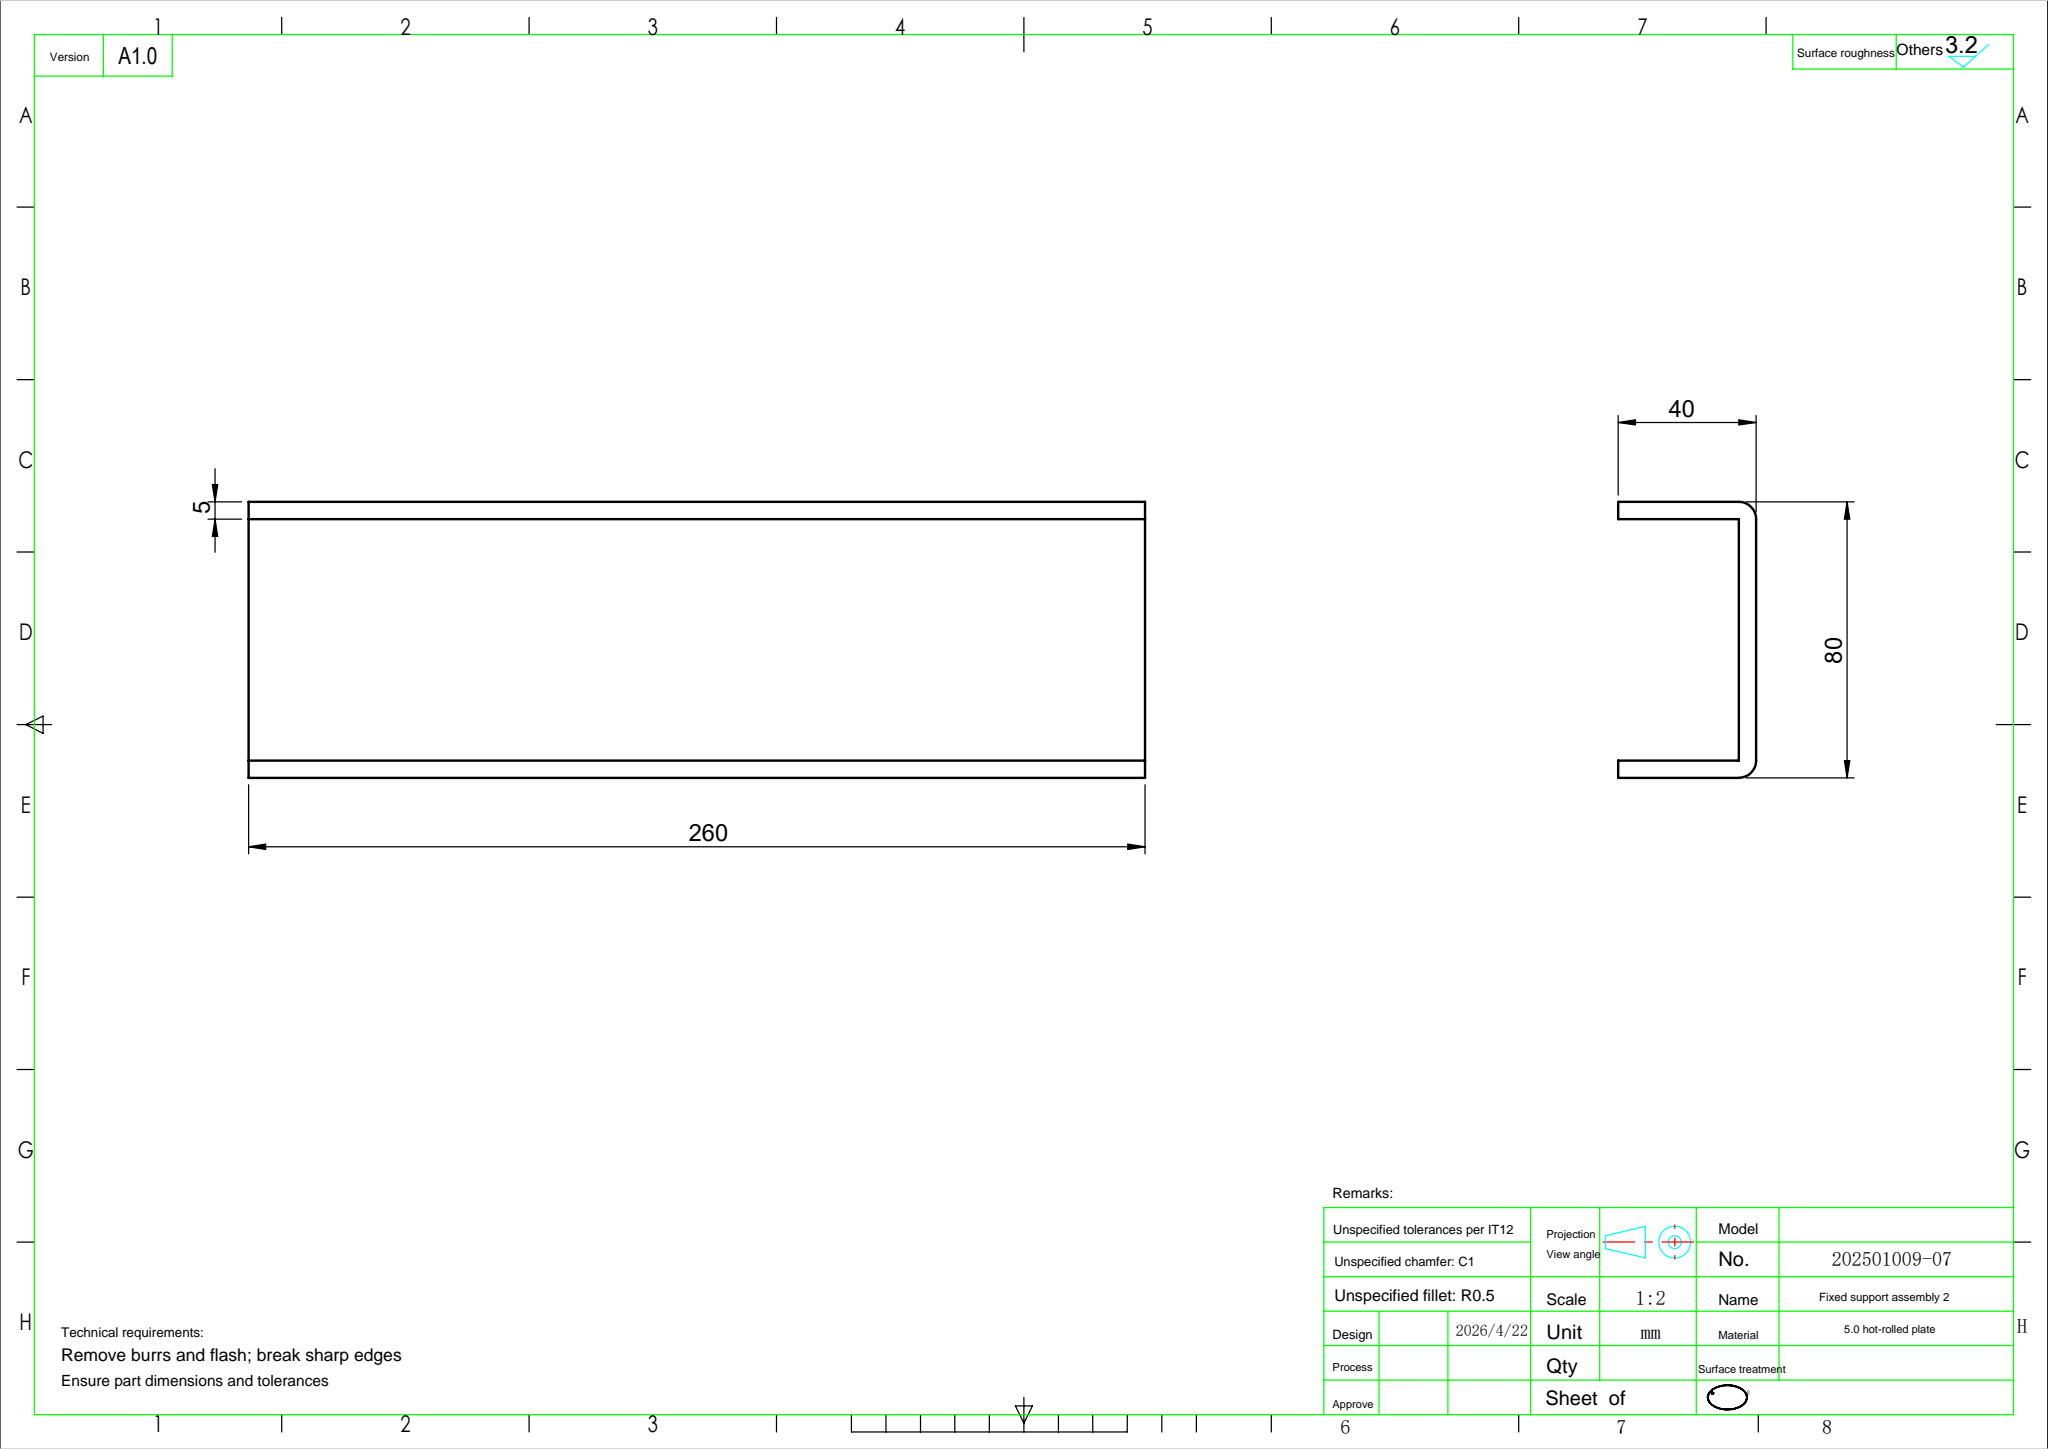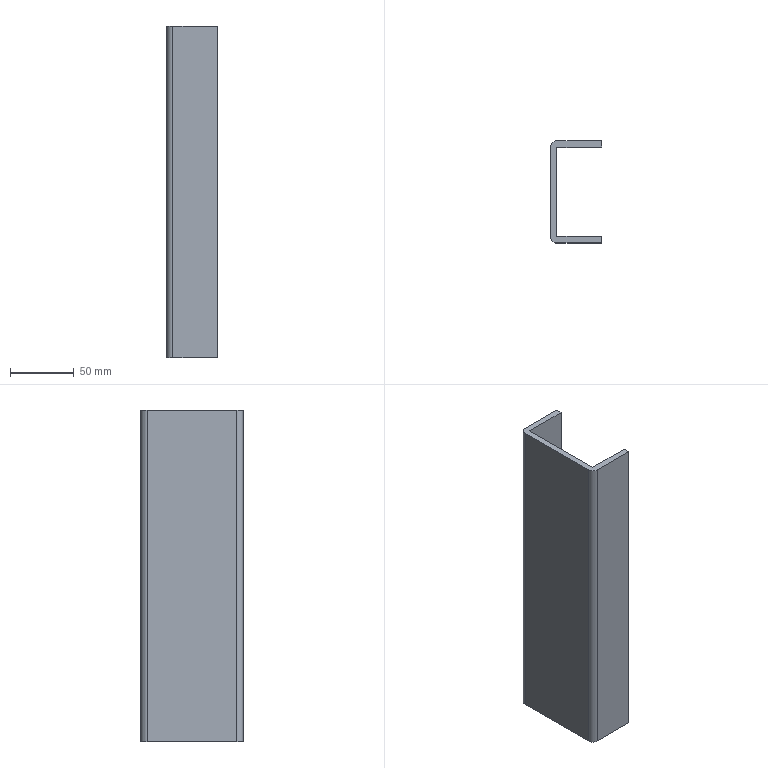Part | SolidWorks | features ExtruThin 1, Fillet 1 | 1 solid | 12 faces | box 40 x 80 x 260 mm | volume 192210 mm3 | plane 10 | cylinder 2 | commonest cylinder face diameters 10 x2
STEP:
#1=CARTESIAN_POINT('',(5.,35.,0.));
#2=VERTEX_POINT('',#1);
#3=CARTESIAN_POINT('',(40.,35.,0.));
#4=VERTEX_POINT('',#3);
#5=CARTESIAN_POINT('',(0.,35.,0.));
#6=DIRECTION('',(1.,0.,0.));
#7=VECTOR('',#6,1000.);
#8=LINE('',#5,#7);
#9=EDGE_CURVE('',#2,#4,#8,.T.);
#10=ORIENTED_EDGE('',*,*,#9,.T.);
#11=CARTESIAN_POINT('',(40.,35.,260.));
#12=VERTEX_POINT('',#11);
#13=CARTESIAN_POINT('',(40.,35.,260.));
#14=DIRECTION('',(0.,0.,-1.));
#15=VECTOR('',#14,1000.);
#16=LINE('',#13,#15);
#17=EDGE_CURVE('',#12,#4,#16,.T.);
#18=ORIENTED_EDGE('',*,*,#17,.F.);
#19=CARTESIAN_POINT('',(5.,35.,260.));
#20=VERTEX_POINT('',#19);
#21=CARTESIAN_POINT('',(0.,35.,260.));
#22=DIRECTION('',(1.,0.,0.));
#23=VECTOR('',#22,1000.);
#24=LINE('',#21,#23);
#25=EDGE_CURVE('',#20,#12,#24,.T.);
#26=ORIENTED_EDGE('',*,*,#25,.F.);
#27=CARTESIAN_POINT('',(5.,35.,260.));
#28=DIRECTION('',(0.,0.,-1.));
#29=VECTOR('',#28,1000.);
#30=LINE('',#27,#29);
#31=EDGE_CURVE('',#20,#2,#30,.T.);
#32=ORIENTED_EDGE('',*,*,#31,.T.);
#33=EDGE_LOOP('',(#10,#18,#26,#32));
#34=FACE_OUTER_BOUND('',#33,.T.);
#35=CARTESIAN_POINT('',(0.,35.,260.));
#36=DIRECTION('',(0.,1.,0.));
#37=DIRECTION('',(0.,0.,1.));
#38=AXIS2_PLACEMENT_3D('',#35,#36,#37);
#39=PLANE('',#38);
#40=ADVANCED_FACE('',(#34),#39,.F.);
#41=CARTESIAN_POINT('',(40.,40.,0.));
#42=VERTEX_POINT('',#41);
#43=CARTESIAN_POINT('',(40.,40.,0.));
#44=DIRECTION('',(0.,-1.,0.));
#45=VECTOR('',#44,1000.);
#46=LINE('',#43,#45);
#47=EDGE_CURVE('',#42,#4,#46,.T.);
#48=ORIENTED_EDGE('',*,*,#47,.F.);
#49=CARTESIAN_POINT('',(40.,40.,260.));
#50=VERTEX_POINT('',#49);
#51=CARTESIAN_POINT('',(40.,40.,260.));
#52=DIRECTION('',(0.,0.,-1.));
#53=VECTOR('',#52,1000.);
#54=LINE('',#51,#53);
#55=EDGE_CURVE('',#50,#42,#54,.T.);
#56=ORIENTED_EDGE('',*,*,#55,.F.);
#57=CARTESIAN_POINT('',(40.,40.,260.));
#58=DIRECTION('',(0.,-1.,0.));
#59=VECTOR('',#58,1000.);
#60=LINE('',#57,#59);
#61=EDGE_CURVE('',#50,#12,#60,.T.);
#62=ORIENTED_EDGE('',*,*,#61,.T.);
#63=ORIENTED_EDGE('',*,*,#17,.T.);
#64=EDGE_LOOP('',(#48,#56,#62,#63));
#65=FACE_OUTER_BOUND('',#64,.T.);
#66=CARTESIAN_POINT('',(40.,40.,260.));
#67=DIRECTION('',(1.,0.,0.));
#68=DIRECTION('',(0.,0.,-1.));
#69=AXIS2_PLACEMENT_3D('',#66,#67,#68);
#70=PLANE('',#69);
#71=ADVANCED_FACE('',(#65),#70,.T.);
#72=CARTESIAN_POINT('',(5.,40.,0.));
#73=VERTEX_POINT('',#72);
#74=CARTESIAN_POINT('',(0.,40.,0.));
#75=DIRECTION('',(1.,0.,0.));
#76=VECTOR('',#75,1000.);
#77=LINE('',#74,#76);
#78=EDGE_CURVE('',#73,#42,#77,.T.);
#79=ORIENTED_EDGE('',*,*,#78,.F.);
#80=CARTESIAN_POINT('',(5.,40.,260.));
#81=VERTEX_POINT('',#80);
#82=CARTESIAN_POINT('',(5.,40.,260.));
#83=DIRECTION('',(0.,0.,1.));
#84=VECTOR('',#83,1000.);
#85=LINE('',#82,#84);
#86=EDGE_CURVE('',#73,#81,#85,.T.);
#87=ORIENTED_EDGE('',*,*,#86,.T.);
#88=CARTESIAN_POINT('',(0.,40.,260.));
#89=DIRECTION('',(1.,0.,0.));
#90=VECTOR('',#89,1000.);
#91=LINE('',#88,#90);
#92=EDGE_CURVE('',#81,#50,#91,.T.);
#93=ORIENTED_EDGE('',*,*,#92,.T.);
#94=ORIENTED_EDGE('',*,*,#55,.T.);
#95=EDGE_LOOP('',(#79,#87,#93,#94));
#96=FACE_OUTER_BOUND('',#95,.T.);
#97=CARTESIAN_POINT('',(0.,40.,260.));
#98=DIRECTION('',(0.,1.,0.));
#99=DIRECTION('',(0.,0.,1.));
#100=AXIS2_PLACEMENT_3D('',#97,#98,#99);
#101=PLANE('',#100);
#102=ADVANCED_FACE('',(#96),#101,.T.);
#103=CARTESIAN_POINT('',(0.,-35.,0.));
#104=VERTEX_POINT('',#103);
#105=CARTESIAN_POINT('',(0.,35.,0.));
#106=VERTEX_POINT('',#105);
#107=CARTESIAN_POINT('',(0.,40.,0.));
#108=DIRECTION('',(0.,1.,0.));
#109=VECTOR('',#108,1000.);
#110=LINE('',#107,#109);
#111=EDGE_CURVE('',#104,#106,#110,.T.);
#112=ORIENTED_EDGE('',*,*,#111,.F.);
#113=CARTESIAN_POINT('',(0.,-35.,260.));
#114=VERTEX_POINT('',#113);
#115=CARTESIAN_POINT('',(0.,-35.,260.));
#116=DIRECTION('',(0.,0.,1.));
#117=VECTOR('',#116,1000.);
#118=LINE('',#115,#117);
#119=EDGE_CURVE('',#104,#114,#118,.T.);
#120=ORIENTED_EDGE('',*,*,#119,.T.);
#121=CARTESIAN_POINT('',(0.,35.,260.));
#122=VERTEX_POINT('',#121);
#123=CARTESIAN_POINT('',(0.,40.,260.));
#124=DIRECTION('',(0.,1.,0.));
#125=VECTOR('',#124,1000.);
#126=LINE('',#123,#125);
#127=EDGE_CURVE('',#114,#122,#126,.T.);
#128=ORIENTED_EDGE('',*,*,#127,.T.);
#129=CARTESIAN_POINT('',(0.,35.,260.));
#130=DIRECTION('',(0.,0.,-1.));
#131=VECTOR('',#130,1000.);
#132=LINE('',#129,#131);
#133=EDGE_CURVE('',#122,#106,#132,.T.);
#134=ORIENTED_EDGE('',*,*,#133,.T.);
#135=EDGE_LOOP('',(#112,#120,#128,#134));
#136=FACE_OUTER_BOUND('',#135,.T.);
#137=CARTESIAN_POINT('',(0.,40.,260.));
#138=DIRECTION('',(-1.,0.,0.));
#139=DIRECTION('',(0.,-1.,0.));
#140=AXIS2_PLACEMENT_3D('',#137,#138,#139);
#141=PLANE('',#140);
#142=ADVANCED_FACE('',(#136),#141,.T.);
#143=CARTESIAN_POINT('',(40.,-40.,260.));
#144=VERTEX_POINT('',#143);
#145=CARTESIAN_POINT('',(5.,-40.,260.));
#146=VERTEX_POINT('',#145);
#147=CARTESIAN_POINT('',(0.,-40.,260.));
#148=DIRECTION('',(-1.,0.,0.));
#149=VECTOR('',#148,1000.);
#150=LINE('',#147,#149);
#151=EDGE_CURVE('',#144,#146,#150,.T.);
#152=ORIENTED_EDGE('',*,*,#151,.T.);
#153=CARTESIAN_POINT('',(5.,-40.,0.));
#154=VERTEX_POINT('',#153);
#155=CARTESIAN_POINT('',(5.,-40.,260.));
#156=DIRECTION('',(0.,0.,-1.));
#157=VECTOR('',#156,1000.);
#158=LINE('',#155,#157);
#159=EDGE_CURVE('',#146,#154,#158,.T.);
#160=ORIENTED_EDGE('',*,*,#159,.T.);
#161=CARTESIAN_POINT('',(40.,-40.,0.));
#162=VERTEX_POINT('',#161);
#163=CARTESIAN_POINT('',(0.,-40.,0.));
#164=DIRECTION('',(-1.,0.,0.));
#165=VECTOR('',#164,1000.);
#166=LINE('',#163,#165);
#167=EDGE_CURVE('',#162,#154,#166,.T.);
#168=ORIENTED_EDGE('',*,*,#167,.F.);
#169=CARTESIAN_POINT('',(40.,-40.,260.));
#170=DIRECTION('',(0.,0.,-1.));
#171=VECTOR('',#170,1000.);
#172=LINE('',#169,#171);
#173=EDGE_CURVE('',#144,#162,#172,.T.);
#174=ORIENTED_EDGE('',*,*,#173,.F.);
#175=EDGE_LOOP('',(#152,#160,#168,#174));
#176=FACE_OUTER_BOUND('',#175,.T.);
#177=CARTESIAN_POINT('',(0.,-40.,260.));
#178=DIRECTION('',(0.,-1.,0.));
#179=DIRECTION('',(0.,0.,-1.));
#180=AXIS2_PLACEMENT_3D('',#177,#178,#179);
#181=PLANE('',#180);
#182=ADVANCED_FACE('',(#176),#181,.T.);
#183=CARTESIAN_POINT('',(40.,-35.,0.));
#184=VERTEX_POINT('',#183);
#185=CARTESIAN_POINT('',(40.,-35.,0.));
#186=DIRECTION('',(0.,-1.,0.));
#187=VECTOR('',#186,1000.);
#188=LINE('',#185,#187);
#189=EDGE_CURVE('',#184,#162,#188,.T.);
#190=ORIENTED_EDGE('',*,*,#189,.F.);
#191=CARTESIAN_POINT('',(40.,-35.,260.));
#192=VERTEX_POINT('',#191);
#193=CARTESIAN_POINT('',(40.,-35.,260.));
#194=DIRECTION('',(0.,0.,-1.));
#195=VECTOR('',#194,1000.);
#196=LINE('',#193,#195);
#197=EDGE_CURVE('',#192,#184,#196,.T.);
#198=ORIENTED_EDGE('',*,*,#197,.F.);
#199=CARTESIAN_POINT('',(40.,-35.,260.));
#200=DIRECTION('',(0.,-1.,0.));
#201=VECTOR('',#200,1000.);
#202=LINE('',#199,#201);
#203=EDGE_CURVE('',#192,#144,#202,.T.);
#204=ORIENTED_EDGE('',*,*,#203,.T.);
#205=ORIENTED_EDGE('',*,*,#173,.T.);
#206=EDGE_LOOP('',(#190,#198,#204,#205));
#207=FACE_OUTER_BOUND('',#206,.T.);
#208=CARTESIAN_POINT('',(40.,-35.,260.));
#209=DIRECTION('',(1.,0.,0.));
#210=DIRECTION('',(0.,0.,-1.));
#211=AXIS2_PLACEMENT_3D('',#208,#209,#210);
#212=PLANE('',#211);
#213=ADVANCED_FACE('',(#207),#212,.T.);
#214=CARTESIAN_POINT('',(5.,-35.,0.));
#215=VERTEX_POINT('',#214);
#216=CARTESIAN_POINT('',(0.,-35.,0.));
#217=DIRECTION('',(-1.,0.,0.));
#218=VECTOR('',#217,1000.);
#219=LINE('',#216,#218);
#220=EDGE_CURVE('',#184,#215,#219,.T.);
#221=ORIENTED_EDGE('',*,*,#220,.T.);
#222=CARTESIAN_POINT('',(5.,-35.,260.));
#223=VERTEX_POINT('',#222);
#224=CARTESIAN_POINT('',(5.,-35.,260.));
#225=DIRECTION('',(0.,0.,-1.));
#226=VECTOR('',#225,1000.);
#227=LINE('',#224,#226);
#228=EDGE_CURVE('',#223,#215,#227,.T.);
#229=ORIENTED_EDGE('',*,*,#228,.F.);
#230=CARTESIAN_POINT('',(0.,-35.,260.));
#231=DIRECTION('',(-1.,0.,0.));
#232=VECTOR('',#231,1000.);
#233=LINE('',#230,#232);
#234=EDGE_CURVE('',#192,#223,#233,.T.);
#235=ORIENTED_EDGE('',*,*,#234,.F.);
#236=ORIENTED_EDGE('',*,*,#197,.T.);
#237=EDGE_LOOP('',(#221,#229,#235,#236));
#238=FACE_OUTER_BOUND('',#237,.T.);
#239=CARTESIAN_POINT('',(0.,-35.,260.));
#240=DIRECTION('',(0.,-1.,0.));
#241=DIRECTION('',(0.,0.,-1.));
#242=AXIS2_PLACEMENT_3D('',#239,#240,#241);
#243=PLANE('',#242);
#244=ADVANCED_FACE('',(#238),#243,.F.);
#245=CARTESIAN_POINT('',(5.,40.,0.));
#246=DIRECTION('',(0.,1.,0.));
#247=VECTOR('',#246,1000.);
#248=LINE('',#245,#247);
#249=EDGE_CURVE('',#215,#2,#248,.T.);
#250=ORIENTED_EDGE('',*,*,#249,.T.);
#251=ORIENTED_EDGE('',*,*,#31,.F.);
#252=CARTESIAN_POINT('',(5.,40.,260.));
#253=DIRECTION('',(0.,1.,0.));
#254=VECTOR('',#253,1000.);
#255=LINE('',#252,#254);
#256=EDGE_CURVE('',#223,#20,#255,.T.);
#257=ORIENTED_EDGE('',*,*,#256,.F.);
#258=ORIENTED_EDGE('',*,*,#228,.T.);
#259=EDGE_LOOP('',(#250,#251,#257,#258));
#260=FACE_OUTER_BOUND('',#259,.T.);
#261=CARTESIAN_POINT('',(5.,40.,260.));
#262=DIRECTION('',(-1.,0.,0.));
#263=DIRECTION('',(0.,-1.,0.));
#264=AXIS2_PLACEMENT_3D('',#261,#262,#263);
#265=PLANE('',#264);
#266=ADVANCED_FACE('',(#260),#265,.F.);
#267=ORIENTED_EDGE('',*,*,#127,.F.);
#268=CARTESIAN_POINT('',(5.,-35.,260.));
#269=DIRECTION('',(0.,0.,1.));
#270=DIRECTION('',(-1.,0.,0.));
#271=AXIS2_PLACEMENT_3D('',#268,#269,#270);
#272=CIRCLE('',#271,5.);
#273=EDGE_CURVE('',#114,#146,#272,.T.);
#274=ORIENTED_EDGE('',*,*,#273,.T.);
#275=ORIENTED_EDGE('',*,*,#151,.F.);
#276=ORIENTED_EDGE('',*,*,#203,.F.);
#277=ORIENTED_EDGE('',*,*,#234,.T.);
#278=ORIENTED_EDGE('',*,*,#256,.T.);
#279=ORIENTED_EDGE('',*,*,#25,.T.);
#280=ORIENTED_EDGE('',*,*,#61,.F.);
#281=ORIENTED_EDGE('',*,*,#92,.F.);
#282=CARTESIAN_POINT('',(5.,35.,260.));
#283=DIRECTION('',(0.,0.,1.));
#284=DIRECTION('',(-1.,0.,0.));
#285=AXIS2_PLACEMENT_3D('',#282,#283,#284);
#286=CIRCLE('',#285,5.);
#287=EDGE_CURVE('',#81,#122,#286,.T.);
#288=ORIENTED_EDGE('',*,*,#287,.T.);
#289=EDGE_LOOP('',(#267,#274,#275,#276,#277,#278,#279,#280,#281,#288));
#290=FACE_OUTER_BOUND('',#289,.T.);
#291=CARTESIAN_POINT('',(0.,0.,260.));
#292=DIRECTION('',(0.,0.,-1.));
#293=DIRECTION('',(-1.,0.,0.));
#294=AXIS2_PLACEMENT_3D('',#291,#292,#293);
#295=PLANE('',#294);
#296=ADVANCED_FACE('',(#290),#295,.F.);
#297=ORIENTED_EDGE('',*,*,#167,.T.);
#298=CARTESIAN_POINT('',(5.,-35.,0.));
#299=DIRECTION('',(0.,0.,-1.));
#300=DIRECTION('',(-1.,0.,0.));
#301=AXIS2_PLACEMENT_3D('',#298,#299,#300);
#302=CIRCLE('',#301,5.);
#303=EDGE_CURVE('',#154,#104,#302,.T.);
#304=ORIENTED_EDGE('',*,*,#303,.T.);
#305=ORIENTED_EDGE('',*,*,#111,.T.);
#306=CARTESIAN_POINT('',(5.,35.,0.));
#307=DIRECTION('',(0.,0.,-1.));
#308=DIRECTION('',(-1.,0.,0.));
#309=AXIS2_PLACEMENT_3D('',#306,#307,#308);
#310=CIRCLE('',#309,5.);
#311=EDGE_CURVE('',#106,#73,#310,.T.);
#312=ORIENTED_EDGE('',*,*,#311,.T.);
#313=ORIENTED_EDGE('',*,*,#78,.T.);
#314=ORIENTED_EDGE('',*,*,#47,.T.);
#315=ORIENTED_EDGE('',*,*,#9,.F.);
#316=ORIENTED_EDGE('',*,*,#249,.F.);
#317=ORIENTED_EDGE('',*,*,#220,.F.);
#318=ORIENTED_EDGE('',*,*,#189,.T.);
#319=EDGE_LOOP('',(#297,#304,#305,#312,#313,#314,#315,#316,#317,#318));
#320=FACE_OUTER_BOUND('',#319,.T.);
#321=CARTESIAN_POINT('',(0.,0.,0.));
#322=DIRECTION('',(0.,0.,-1.));
#323=DIRECTION('',(-1.,0.,0.));
#324=AXIS2_PLACEMENT_3D('',#321,#322,#323);
#325=PLANE('',#324);
#326=ADVANCED_FACE('',(#320),#325,.T.);
#327=ORIENTED_EDGE('',*,*,#273,.F.);
#328=ORIENTED_EDGE('',*,*,#119,.F.);
#329=ORIENTED_EDGE('',*,*,#303,.F.);
#330=ORIENTED_EDGE('',*,*,#159,.F.);
#331=EDGE_LOOP('',(#327,#328,#329,#330));
#332=FACE_OUTER_BOUND('',#331,.T.);
#333=CARTESIAN_POINT('',(5.,-35.,260.));
#334=DIRECTION('',(0.,0.,-1.));
#335=DIRECTION('',(-1.,0.,0.));
#336=AXIS2_PLACEMENT_3D('',#333,#334,#335);
#337=CYLINDRICAL_SURFACE('',#336,5.);
#338=ADVANCED_FACE('',(#332),#337,.T.);
#339=ORIENTED_EDGE('',*,*,#287,.F.);
#340=ORIENTED_EDGE('',*,*,#86,.F.);
#341=ORIENTED_EDGE('',*,*,#311,.F.);
#342=ORIENTED_EDGE('',*,*,#133,.F.);
#343=EDGE_LOOP('',(#339,#340,#341,#342));
#344=FACE_OUTER_BOUND('',#343,.T.);
#345=CARTESIAN_POINT('',(5.,35.,260.));
#346=DIRECTION('',(0.,0.,-1.));
#347=DIRECTION('',(-1.,0.,0.));
#348=AXIS2_PLACEMENT_3D('',#345,#346,#347);
#349=CYLINDRICAL_SURFACE('',#348,5.);
#350=ADVANCED_FACE('',(#344),#349,.T.);
#351=CLOSED_SHELL('',(#40,#71,#102,#142,#182,#213,#244,#266,#296,#326,#338,#350));
#352=MANIFOLD_SOLID_BREP('',#351);
#353=CARTESIAN_POINT('',(0.,0.,0.));
#354=DIRECTION('',(0.,0.,1.));
#355=DIRECTION('',(1.,0.,0.));
#356=AXIS2_PLACEMENT_3D('',#353,#354,#355);
#357=(LENGTH_UNIT()NAMED_UNIT(*)SI_UNIT(.MILLI.,.METRE.));
#358=UNCERTAINTY_MEASURE_WITH_UNIT(LENGTH_MEASURE(0.00001),#357,'','');
#359=(NAMED_UNIT(*)PLANE_ANGLE_UNIT()SI_UNIT($,.RADIAN.));
#360=(NAMED_UNIT(*)SI_UNIT($,.STERADIAN.)SOLID_ANGLE_UNIT());
#361=(GEOMETRIC_REPRESENTATION_CONTEXT(3)GLOBAL_UNCERTAINTY_ASSIGNED_CONTEXT((#358))GLOBAL_UNIT_ASSIGNED_CONTEXT((#357,#359,#360))REPRESENTATION_CONTEXT('',''));
#362=ADVANCED_BREP_SHAPE_REPRESENTATION('',(#352,#356),#361);